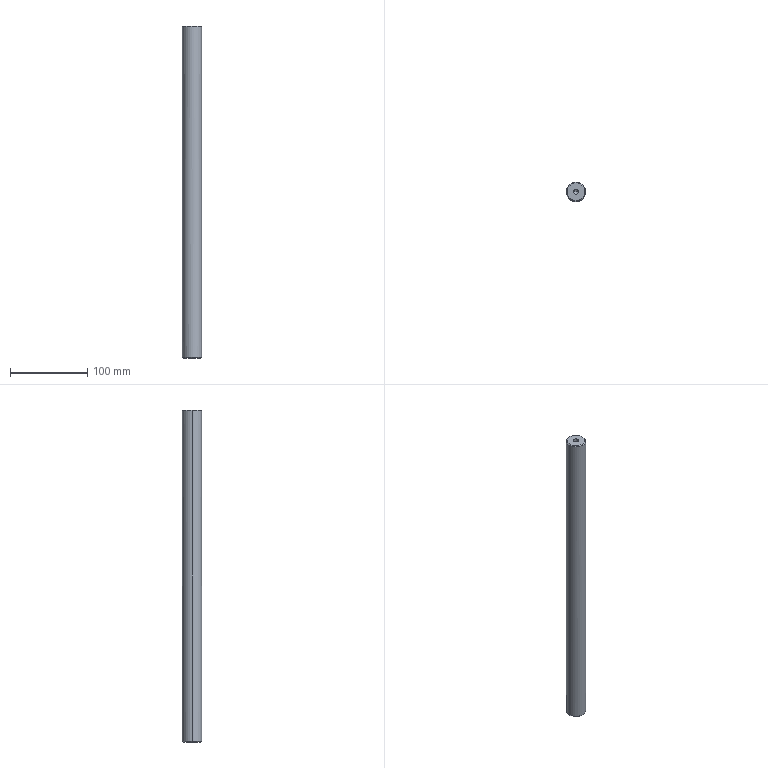Part | STEP file | fBY02F02M-00-20A | 1 solid | 16 faces | box 25 x 25 x 430 mm | volume 209515 mm3 | cone 8 | cylinder 6 | plane 2 | commonest cylinder face diameters 6.8 x4 25 x2
STEP:
#1=CARTESIAN_POINT('',(0.,0.,0.));
#2=DIRECTION('',(0.,0.,1.));
#3=DIRECTION('',(1.,0.,0.));
#4=AXIS2_PLACEMENT_3D('',#1,#2,#3);
#5=CARTESIAN_POINT('',(0.,12.5,429.));
#6=VERTEX_POINT('',#5);
#7=CARTESIAN_POINT('',(12.5,0.,429.));
#8=VERTEX_POINT('',#7);
#9=CARTESIAN_POINT('',(0.,0.,429.));
#10=DIRECTION('',(0.,0.,-1.));
#11=DIRECTION('',(-1.,0.,0.));
#12=AXIS2_PLACEMENT_3D('',#9,#10,#11);
#13=CIRCLE('',#12,12.5);
#14=CARTESIAN_POINT('',(0.,0.,430.));
#15=DIRECTION('',(0.,0.,-1.));
#16=DIRECTION('',(-1.,0.,0.));
#17=AXIS2_PLACEMENT_3D('',#14,#15,#16);
#18=CYLINDRICAL_SURFACE('',#17,12.5);
#19=CARTESIAN_POINT('',(0.,1.));
#20=DIRECTION('',(1.,0.));
#21=VECTOR('',#20,1.);
#22=LINE('',#19,#21);
#23=(GEOMETRIC_REPRESENTATION_CONTEXT(2)PARAMETRIC_REPRESENTATION_CONTEXT()REPRESENTATION_CONTEXT('',''));
#24=DEFINITIONAL_REPRESENTATION('',(#22),#23);
#25=PCURVE('',#18,#24);
#26=CARTESIAN_POINT('',(0.,0.,429.));
#27=DIRECTION('',(0.,0.,-1.));
#28=DIRECTION('',(0.,1.,0.));
#29=AXIS2_PLACEMENT_3D('',#26,#27,#28);
#30=CONICAL_SURFACE('',#29,12.5,0.7854);
#31=CARTESIAN_POINT('',(-1.571,0.));
#32=DIRECTION('',(1.,0.));
#33=VECTOR('',#32,1.);
#34=LINE('',#31,#33);
#35=(GEOMETRIC_REPRESENTATION_CONTEXT(2)PARAMETRIC_REPRESENTATION_CONTEXT()REPRESENTATION_CONTEXT('',''));
#36=DEFINITIONAL_REPRESENTATION('',(#34),#35);
#37=PCURVE('',#30,#36);
#38=SURFACE_CURVE('',#13,(#25,#37),.PCURVE_S1.);
#39=EDGE_CURVE('',#6,#8,#38,.T.);
#40=ORIENTED_EDGE('',*,*,#39,.T.);
#41=CARTESIAN_POINT('',(12.5,0.,1.));
#42=VERTEX_POINT('',#41);
#43=CARTESIAN_POINT('',(12.5,0.,430.));
#44=DIRECTION('',(0.,0.,-1.));
#45=VECTOR('',#44,1.);
#46=LINE('',#43,#45);
#47=CARTESIAN_POINT('',(3.142,0.));
#48=DIRECTION('',(0.,1.));
#49=VECTOR('',#48,1.);
#50=LINE('',#47,#49);
#51=(GEOMETRIC_REPRESENTATION_CONTEXT(2)PARAMETRIC_REPRESENTATION_CONTEXT()REPRESENTATION_CONTEXT('',''));
#52=DEFINITIONAL_REPRESENTATION('',(#50),#51);
#53=PCURVE('',#18,#52);
#54=CARTESIAN_POINT('',(0.,0.,430.));
#55=DIRECTION('',(0.,0.,-1.));
#56=DIRECTION('',(-1.,0.,0.));
#57=AXIS2_PLACEMENT_3D('',#54,#55,#56);
#58=CYLINDRICAL_SURFACE('',#57,12.5);
#59=CARTESIAN_POINT('',(3.142,0.));
#60=DIRECTION('',(0.,1.));
#61=VECTOR('',#60,1.);
#62=LINE('',#59,#61);
#63=(GEOMETRIC_REPRESENTATION_CONTEXT(2)PARAMETRIC_REPRESENTATION_CONTEXT()REPRESENTATION_CONTEXT('',''));
#64=DEFINITIONAL_REPRESENTATION('',(#62),#63);
#65=PCURVE('',#58,#64);
#66=SURFACE_CURVE('',#46,(#53,#65),.PCURVE_S1.);
#67=EDGE_CURVE('',#8,#42,#66,.T.);
#68=ORIENTED_EDGE('',*,*,#67,.T.);
#69=CARTESIAN_POINT('',(-12.5,0.,1.));
#70=VERTEX_POINT('',#69);
#71=CARTESIAN_POINT('',(0.,0.,1.));
#72=DIRECTION('',(0.,0.,1.));
#73=DIRECTION('',(-1.,0.,0.));
#74=AXIS2_PLACEMENT_3D('',#71,#72,#73);
#75=CIRCLE('',#74,12.5);
#76=CARTESIAN_POINT('',(6.283,429.));
#77=DIRECTION('',(-1.,0.));
#78=VECTOR('',#77,1.);
#79=LINE('',#76,#78);
#80=(GEOMETRIC_REPRESENTATION_CONTEXT(2)PARAMETRIC_REPRESENTATION_CONTEXT()REPRESENTATION_CONTEXT('',''));
#81=DEFINITIONAL_REPRESENTATION('',(#79),#80);
#82=PCURVE('',#18,#81);
#83=CARTESIAN_POINT('',(0.,0.,1.));
#84=DIRECTION('',(0.,0.,1.));
#85=DIRECTION('',(1.,0.,0.));
#86=AXIS2_PLACEMENT_3D('',#83,#84,#85);
#87=CONICAL_SURFACE('',#86,12.5,0.7854);
#88=CARTESIAN_POINT('',(-3.142,0.));
#89=DIRECTION('',(1.,0.));
#90=VECTOR('',#89,1.);
#91=LINE('',#88,#90);
#92=(GEOMETRIC_REPRESENTATION_CONTEXT(2)PARAMETRIC_REPRESENTATION_CONTEXT()REPRESENTATION_CONTEXT('',''));
#93=DEFINITIONAL_REPRESENTATION('',(#91),#92);
#94=PCURVE('',#87,#93);
#95=SURFACE_CURVE('',#75,(#82,#94),.PCURVE_S1.);
#96=EDGE_CURVE('',#42,#70,#95,.T.);
#97=ORIENTED_EDGE('',*,*,#96,.T.);
#98=CARTESIAN_POINT('',(-12.5,0.,429.));
#99=VERTEX_POINT('',#98);
#100=CARTESIAN_POINT('',(-12.5,0.,430.));
#101=DIRECTION('',(0.,0.,-1.));
#102=VECTOR('',#101,1.);
#103=LINE('',#100,#102);
#104=CARTESIAN_POINT('',(0.,0.));
#105=DIRECTION('',(0.,1.));
#106=VECTOR('',#105,1.);
#107=LINE('',#104,#106);
#108=(GEOMETRIC_REPRESENTATION_CONTEXT(2)PARAMETRIC_REPRESENTATION_CONTEXT()REPRESENTATION_CONTEXT('',''));
#109=DEFINITIONAL_REPRESENTATION('',(#107),#108);
#110=PCURVE('',#18,#109);
#111=CARTESIAN_POINT('',(6.283,0.));
#112=DIRECTION('',(0.,1.));
#113=VECTOR('',#112,1.);
#114=LINE('',#111,#113);
#115=(GEOMETRIC_REPRESENTATION_CONTEXT(2)PARAMETRIC_REPRESENTATION_CONTEXT()REPRESENTATION_CONTEXT('',''));
#116=DEFINITIONAL_REPRESENTATION('',(#114),#115);
#117=PCURVE('',#58,#116);
#118=SURFACE_CURVE('',#103,(#110,#117),.PCURVE_S1.);
#119=EDGE_CURVE('',#99,#70,#118,.T.);
#120=ORIENTED_EDGE('',*,*,#119,.F.);
#121=CARTESIAN_POINT('',(0.,0.,429.));
#122=DIRECTION('',(0.,0.,-1.));
#123=DIRECTION('',(-1.,0.,0.));
#124=AXIS2_PLACEMENT_3D('',#121,#122,#123);
#125=CIRCLE('',#124,12.5);
#126=CARTESIAN_POINT('',(0.,1.));
#127=DIRECTION('',(1.,0.));
#128=VECTOR('',#127,1.);
#129=LINE('',#126,#128);
#130=(GEOMETRIC_REPRESENTATION_CONTEXT(2)PARAMETRIC_REPRESENTATION_CONTEXT()REPRESENTATION_CONTEXT('',''));
#131=DEFINITIONAL_REPRESENTATION('',(#129),#130);
#132=PCURVE('',#18,#131);
#133=CARTESIAN_POINT('',(0.,0.,429.));
#134=DIRECTION('',(0.,0.,-1.));
#135=DIRECTION('',(0.,1.,0.));
#136=AXIS2_PLACEMENT_3D('',#133,#134,#135);
#137=CONICAL_SURFACE('',#136,12.5,0.7854);
#138=CARTESIAN_POINT('',(4.712,0.));
#139=DIRECTION('',(1.,0.));
#140=VECTOR('',#139,1.);
#141=LINE('',#138,#140);
#142=(GEOMETRIC_REPRESENTATION_CONTEXT(2)PARAMETRIC_REPRESENTATION_CONTEXT()REPRESENTATION_CONTEXT('',''));
#143=DEFINITIONAL_REPRESENTATION('',(#141),#142);
#144=PCURVE('',#137,#143);
#145=SURFACE_CURVE('',#125,(#132,#144),.PCURVE_S1.);
#146=EDGE_CURVE('',#99,#6,#145,.T.);
#147=ORIENTED_EDGE('',*,*,#146,.T.);
#148=EDGE_LOOP('',(#40,#68,#97,#120,#147));
#149=FACE_BOUND('',#148,.T.);
#150=ADVANCED_FACE('',(#149),#18,.T.);
#151=CARTESIAN_POINT('',(11.5,0.,0.));
#152=VERTEX_POINT('',#151);
#153=CARTESIAN_POINT('',(-11.5,0.,0.));
#154=VERTEX_POINT('',#153);
#155=CARTESIAN_POINT('',(0.,0.,0.));
#156=DIRECTION('',(0.,0.,1.));
#157=DIRECTION('',(1.,0.,0.));
#158=AXIS2_PLACEMENT_3D('',#155,#156,#157);
#159=CIRCLE('',#158,11.5);
#160=CARTESIAN_POINT('',(0.,-1.));
#161=DIRECTION('',(1.,0.));
#162=VECTOR('',#161,1.);
#163=LINE('',#160,#162);
#164=(GEOMETRIC_REPRESENTATION_CONTEXT(2)PARAMETRIC_REPRESENTATION_CONTEXT()REPRESENTATION_CONTEXT('',''));
#165=DEFINITIONAL_REPRESENTATION('',(#163),#164);
#166=PCURVE('',#87,#165);
#167=CARTESIAN_POINT('',(0.,0.,0.));
#168=DIRECTION('',(0.,0.,1.));
#169=DIRECTION('',(1.,0.,0.));
#170=AXIS2_PLACEMENT_3D('',#167,#168,#169);
#171=PLANE('',#170);
#172=CARTESIAN_POINT('',(0.,0.));
#173=DIRECTION('',(1.,0.));
#174=AXIS2_PLACEMENT_2D('',#172,#173);
#175=CIRCLE('',#174,11.5);
#176=(GEOMETRIC_REPRESENTATION_CONTEXT(2)PARAMETRIC_REPRESENTATION_CONTEXT()REPRESENTATION_CONTEXT('',''));
#177=DEFINITIONAL_REPRESENTATION('',(#175),#176);
#178=PCURVE('',#171,#177);
#179=SURFACE_CURVE('',#159,(#166,#178),.PCURVE_S1.);
#180=EDGE_CURVE('',#152,#154,#179,.T.);
#181=ORIENTED_EDGE('',*,*,#180,.T.);
#182=CARTESIAN_POINT('',(-12.5,0.,1.));
#183=DIRECTION('',(-0.7071,0.,0.7071));
#184=VECTOR('',#183,1.);
#185=LINE('',#182,#184);
#186=CARTESIAN_POINT('',(3.142,0.));
#187=DIRECTION('',(0.,1.));
#188=VECTOR('',#187,1.);
#189=LINE('',#186,#188);
#190=(GEOMETRIC_REPRESENTATION_CONTEXT(2)PARAMETRIC_REPRESENTATION_CONTEXT()REPRESENTATION_CONTEXT('',''));
#191=DEFINITIONAL_REPRESENTATION('',(#189),#190);
#192=PCURVE('',#87,#191);
#193=CARTESIAN_POINT('',(0.,0.,1.));
#194=DIRECTION('',(0.,0.,1.));
#195=DIRECTION('',(1.,0.,0.));
#196=AXIS2_PLACEMENT_3D('',#193,#194,#195);
#197=CONICAL_SURFACE('',#196,12.5,0.7854);
#198=CARTESIAN_POINT('',(3.142,0.));
#199=DIRECTION('',(0.,1.));
#200=VECTOR('',#199,1.);
#201=LINE('',#198,#200);
#202=(GEOMETRIC_REPRESENTATION_CONTEXT(2)PARAMETRIC_REPRESENTATION_CONTEXT()REPRESENTATION_CONTEXT('',''));
#203=DEFINITIONAL_REPRESENTATION('',(#201),#202);
#204=PCURVE('',#197,#203);
#205=SURFACE_CURVE('',#185,(#192,#204),.PCURVE_S1.);
#206=EDGE_CURVE('',#154,#70,#205,.T.);
#207=ORIENTED_EDGE('',*,*,#206,.T.);
#208=ORIENTED_EDGE('',*,*,#96,.F.);
#209=CARTESIAN_POINT('',(12.5,0.,1.));
#210=DIRECTION('',(0.7071,0.,0.7071));
#211=VECTOR('',#210,1.);
#212=LINE('',#209,#211);
#213=CARTESIAN_POINT('',(0.,0.));
#214=DIRECTION('',(0.,1.));
#215=VECTOR('',#214,1.);
#216=LINE('',#213,#215);
#217=(GEOMETRIC_REPRESENTATION_CONTEXT(2)PARAMETRIC_REPRESENTATION_CONTEXT()REPRESENTATION_CONTEXT('',''));
#218=DEFINITIONAL_REPRESENTATION('',(#216),#217);
#219=PCURVE('',#87,#218);
#220=CARTESIAN_POINT('',(6.283,0.));
#221=DIRECTION('',(0.,1.));
#222=VECTOR('',#221,1.);
#223=LINE('',#220,#222);
#224=(GEOMETRIC_REPRESENTATION_CONTEXT(2)PARAMETRIC_REPRESENTATION_CONTEXT()REPRESENTATION_CONTEXT('',''));
#225=DEFINITIONAL_REPRESENTATION('',(#223),#224);
#226=PCURVE('',#197,#225);
#227=SURFACE_CURVE('',#212,(#219,#226),.PCURVE_S1.);
#228=EDGE_CURVE('',#152,#42,#227,.T.);
#229=ORIENTED_EDGE('',*,*,#228,.F.);
#230=EDGE_LOOP('',(#181,#207,#208,#229));
#231=FACE_BOUND('',#230,.T.);
#232=ADVANCED_FACE('',(#231),#87,.T.);
#233=CARTESIAN_POINT('',(0.,11.5,430.));
#234=VERTEX_POINT('',#233);
#235=CARTESIAN_POINT('',(0.,-11.5,430.));
#236=VERTEX_POINT('',#235);
#237=CARTESIAN_POINT('',(0.,0.,430.));
#238=DIRECTION('',(0.,0.,-1.));
#239=DIRECTION('',(0.,1.,0.));
#240=AXIS2_PLACEMENT_3D('',#237,#238,#239);
#241=CIRCLE('',#240,11.5);
#242=CARTESIAN_POINT('',(0.,-1.));
#243=DIRECTION('',(1.,0.));
#244=VECTOR('',#243,1.);
#245=LINE('',#242,#244);
#246=(GEOMETRIC_REPRESENTATION_CONTEXT(2)PARAMETRIC_REPRESENTATION_CONTEXT()REPRESENTATION_CONTEXT('',''));
#247=DEFINITIONAL_REPRESENTATION('',(#245),#246);
#248=PCURVE('',#30,#247);
#249=CARTESIAN_POINT('',(0.,0.,430.));
#250=DIRECTION('',(0.,0.,1.));
#251=DIRECTION('',(1.,0.,0.));
#252=AXIS2_PLACEMENT_3D('',#249,#250,#251);
#253=PLANE('',#252);
#254=CARTESIAN_POINT('',(0.,11.5));
#255=CARTESIAN_POINT('',(19.919,11.5));
#256=CARTESIAN_POINT('',(9.959,-5.75));
#257=CARTESIAN_POINT('',(0.,-23.));
#258=CARTESIAN_POINT('',(-9.959,-5.75));
#259=CARTESIAN_POINT('',(-19.919,11.5));
#260=CARTESIAN_POINT('',(0.,11.5));
#261=(BOUNDED_CURVE()B_SPLINE_CURVE(2,(#254,#255,#256,#257,#258,#259,#260),.UNSPECIFIED.,.T.,.F.)B_SPLINE_CURVE_WITH_KNOTS((1,2,2,2,2,1),(-2.094,0.,2.094,4.189,6.283,8.378),.UNSPECIFIED.)CURVE()GEOMETRIC_REPRESENTATION_ITEM()RATIONAL_B_SPLINE_CURVE((1.,0.5,1.,0.5,1.,0.5,1.))REPRESENTATION_ITEM(''));
#262=(GEOMETRIC_REPRESENTATION_CONTEXT(2)PARAMETRIC_REPRESENTATION_CONTEXT()REPRESENTATION_CONTEXT('',''));
#263=DEFINITIONAL_REPRESENTATION('',(#261),#262);
#264=PCURVE('',#253,#263);
#265=SURFACE_CURVE('',#241,(#248,#264),.PCURVE_S1.);
#266=EDGE_CURVE('',#234,#236,#265,.T.);
#267=ORIENTED_EDGE('',*,*,#266,.T.);
#268=CARTESIAN_POINT('',(0.,-12.5,429.));
#269=VERTEX_POINT('',#268);
#270=CARTESIAN_POINT('',(0.,-12.5,429.));
#271=DIRECTION('',(0.,-0.7071,-0.7071));
#272=VECTOR('',#271,1.);
#273=LINE('',#270,#272);
#274=CARTESIAN_POINT('',(3.142,0.));
#275=DIRECTION('',(0.,1.));
#276=VECTOR('',#275,1.);
#277=LINE('',#274,#276);
#278=(GEOMETRIC_REPRESENTATION_CONTEXT(2)PARAMETRIC_REPRESENTATION_CONTEXT()REPRESENTATION_CONTEXT('',''));
#279=DEFINITIONAL_REPRESENTATION('',(#277),#278);
#280=PCURVE('',#30,#279);
#281=CARTESIAN_POINT('',(3.142,0.));
#282=DIRECTION('',(0.,1.));
#283=VECTOR('',#282,1.);
#284=LINE('',#281,#283);
#285=(GEOMETRIC_REPRESENTATION_CONTEXT(2)PARAMETRIC_REPRESENTATION_CONTEXT()REPRESENTATION_CONTEXT('',''));
#286=DEFINITIONAL_REPRESENTATION('',(#284),#285);
#287=PCURVE('',#137,#286);
#288=SURFACE_CURVE('',#273,(#280,#287),.PCURVE_S1.);
#289=EDGE_CURVE('',#236,#269,#288,.T.);
#290=ORIENTED_EDGE('',*,*,#289,.T.);
#291=CARTESIAN_POINT('',(0.,0.,429.));
#292=DIRECTION('',(0.,0.,-1.));
#293=DIRECTION('',(-1.,0.,0.));
#294=AXIS2_PLACEMENT_3D('',#291,#292,#293);
#295=CIRCLE('',#294,12.5);
#296=CARTESIAN_POINT('',(-1.571,0.));
#297=DIRECTION('',(1.,0.));
#298=VECTOR('',#297,1.);
#299=LINE('',#296,#298);
#300=(GEOMETRIC_REPRESENTATION_CONTEXT(2)PARAMETRIC_REPRESENTATION_CONTEXT()REPRESENTATION_CONTEXT('',''));
#301=DEFINITIONAL_REPRESENTATION('',(#299),#300);
#302=PCURVE('',#30,#301);
#303=CARTESIAN_POINT('',(0.,1.));
#304=DIRECTION('',(1.,0.));
#305=VECTOR('',#304,1.);
#306=LINE('',#303,#305);
#307=(GEOMETRIC_REPRESENTATION_CONTEXT(2)PARAMETRIC_REPRESENTATION_CONTEXT()REPRESENTATION_CONTEXT('',''));
#308=DEFINITIONAL_REPRESENTATION('',(#306),#307);
#309=PCURVE('',#58,#308);
#310=SURFACE_CURVE('',#295,(#302,#309),.PCURVE_S1.);
#311=EDGE_CURVE('',#8,#269,#310,.T.);
#312=ORIENTED_EDGE('',*,*,#311,.F.);
#313=ORIENTED_EDGE('',*,*,#39,.F.);
#314=CARTESIAN_POINT('',(0.,12.5,429.));
#315=DIRECTION('',(0.,0.7071,-0.7071));
#316=VECTOR('',#315,1.);
#317=LINE('',#314,#316);
#318=CARTESIAN_POINT('',(0.,0.));
#319=DIRECTION('',(0.,1.));
#320=VECTOR('',#319,1.);
#321=LINE('',#318,#320);
#322=(GEOMETRIC_REPRESENTATION_CONTEXT(2)PARAMETRIC_REPRESENTATION_CONTEXT()REPRESENTATION_CONTEXT('',''));
#323=DEFINITIONAL_REPRESENTATION('',(#321),#322);
#324=PCURVE('',#30,#323);
#325=CARTESIAN_POINT('',(6.283,0.));
#326=DIRECTION('',(0.,1.));
#327=VECTOR('',#326,1.);
#328=LINE('',#325,#327);
#329=(GEOMETRIC_REPRESENTATION_CONTEXT(2)PARAMETRIC_REPRESENTATION_CONTEXT()REPRESENTATION_CONTEXT('',''));
#330=DEFINITIONAL_REPRESENTATION('',(#328),#329);
#331=PCURVE('',#137,#330);
#332=SURFACE_CURVE('',#317,(#324,#331),.PCURVE_S1.);
#333=EDGE_CURVE('',#234,#6,#332,.T.);
#334=ORIENTED_EDGE('',*,*,#333,.F.);
#335=EDGE_LOOP('',(#267,#290,#312,#313,#334));
#336=FACE_BOUND('',#335,.T.);
#337=ADVANCED_FACE('',(#336),#30,.T.);
#338=CARTESIAN_POINT('',(-3.4,0.,19.75));
#339=VERTEX_POINT('',#338);
#340=CARTESIAN_POINT('',(-3.4,0.,0.));
#341=VERTEX_POINT('',#340);
#342=CARTESIAN_POINT('',(-3.4,0.,0.));
#343=DIRECTION('',(0.,0.,-1.));
#344=VECTOR('',#343,1.);
#345=LINE('',#342,#344);
#346=CARTESIAN_POINT('',(0.,0.,0.));
#347=DIRECTION('',(0.,0.,-1.));
#348=DIRECTION('',(-1.,0.,0.));
#349=AXIS2_PLACEMENT_3D('',#346,#347,#348);
#350=CYLINDRICAL_SURFACE('',#349,3.4);
#351=CARTESIAN_POINT('',(6.283,0.));
#352=DIRECTION('',(0.,1.));
#353=VECTOR('',#352,1.);
#354=LINE('',#351,#353);
#355=(GEOMETRIC_REPRESENTATION_CONTEXT(2)PARAMETRIC_REPRESENTATION_CONTEXT()REPRESENTATION_CONTEXT('',''));
#356=DEFINITIONAL_REPRESENTATION('',(#354),#355);
#357=PCURVE('',#350,#356);
#358=CARTESIAN_POINT('',(0.,0.,0.));
#359=DIRECTION('',(0.,0.,-1.));
#360=DIRECTION('',(-1.,0.,0.));
#361=AXIS2_PLACEMENT_3D('',#358,#359,#360);
#362=CYLINDRICAL_SURFACE('',#361,3.4);
#363=CARTESIAN_POINT('',(0.,0.));
#364=DIRECTION('',(0.,1.));
#365=VECTOR('',#364,1.);
#366=LINE('',#363,#365);
#367=(GEOMETRIC_REPRESENTATION_CONTEXT(2)PARAMETRIC_REPRESENTATION_CONTEXT()REPRESENTATION_CONTEXT('',''));
#368=DEFINITIONAL_REPRESENTATION('',(#366),#367);
#369=PCURVE('',#362,#368);
#370=SURFACE_CURVE('',#345,(#357,#369),.PCURVE_S1.);
#371=EDGE_CURVE('',#339,#341,#370,.T.);
#372=ORIENTED_EDGE('',*,*,#371,.T.);
#373=CARTESIAN_POINT('',(3.4,0.,0.));
#374=VERTEX_POINT('',#373);
#375=CARTESIAN_POINT('',(0.,0.,0.));
#376=DIRECTION('',(0.,0.,-1.));
#377=DIRECTION('',(-1.,0.,0.));
#378=AXIS2_PLACEMENT_3D('',#375,#376,#377);
#379=CIRCLE('',#378,3.4);
#380=CARTESIAN_POINT('',(0.,0.));
#381=DIRECTION('',(1.,0.));
#382=VECTOR('',#381,1.);
#383=LINE('',#380,#382);
#384=(GEOMETRIC_REPRESENTATION_CONTEXT(2)PARAMETRIC_REPRESENTATION_CONTEXT()REPRESENTATION_CONTEXT('',''));
#385=DEFINITIONAL_REPRESENTATION('',(#383),#384);
#386=PCURVE('',#350,#385);
#387=CARTESIAN_POINT('',(-3.4,0.));
#388=CARTESIAN_POINT('',(-3.4,5.889));
#389=CARTESIAN_POINT('',(1.7,2.944));
#390=CARTESIAN_POINT('',(6.8,0.));
#391=CARTESIAN_POINT('',(1.7,-2.944));
#392=CARTESIAN_POINT('',(-3.4,-5.889));
#393=CARTESIAN_POINT('',(-3.4,0.));
#394=(BOUNDED_CURVE()B_SPLINE_CURVE(2,(#387,#388,#389,#390,#391,#392,#393),.UNSPECIFIED.,.T.,.F.)B_SPLINE_CURVE_WITH_KNOTS((1,2,2,2,2,1),(-2.094,0.,2.094,4.189,6.283,8.378),.UNSPECIFIED.)CURVE()GEOMETRIC_REPRESENTATION_ITEM()RATIONAL_B_SPLINE_CURVE((1.,0.5,1.,0.5,1.,0.5,1.))REPRESENTATION_ITEM(''));
#395=(GEOMETRIC_REPRESENTATION_CONTEXT(2)PARAMETRIC_REPRESENTATION_CONTEXT()REPRESENTATION_CONTEXT('',''));
#396=DEFINITIONAL_REPRESENTATION('',(#394),#395);
#397=PCURVE('',#171,#396);
#398=SURFACE_CURVE('',#379,(#386,#397),.PCURVE_S1.);
#399=EDGE_CURVE('',#374,#341,#398,.T.);
#400=ORIENTED_EDGE('',*,*,#399,.F.);
#401=CARTESIAN_POINT('',(3.4,0.,19.75));
#402=VERTEX_POINT('',#401);
#403=CARTESIAN_POINT('',(3.4,0.,0.));
#404=DIRECTION('',(0.,0.,-1.));
#405=VECTOR('',#404,1.);
#406=LINE('',#403,#405);
#407=CARTESIAN_POINT('',(3.142,0.));
#408=DIRECTION('',(0.,1.));
#409=VECTOR('',#408,1.);
#410=LINE('',#407,#409);
#411=(GEOMETRIC_REPRESENTATION_CONTEXT(2)PARAMETRIC_REPRESENTATION_CONTEXT()REPRESENTATION_CONTEXT('',''));
#412=DEFINITIONAL_REPRESENTATION('',(#410),#411);
#413=PCURVE('',#350,#412);
#414=CARTESIAN_POINT('',(3.142,0.));
#415=DIRECTION('',(0.,1.));
#416=VECTOR('',#415,1.);
#417=LINE('',#414,#416);
#418=(GEOMETRIC_REPRESENTATION_CONTEXT(2)PARAMETRIC_REPRESENTATION_CONTEXT()REPRESENTATION_CONTEXT('',''));
#419=DEFINITIONAL_REPRESENTATION('',(#417),#418);
#420=PCURVE('',#362,#419);
#421=SURFACE_CURVE('',#406,(#413,#420),.PCURVE_S1.);
#422=EDGE_CURVE('',#402,#374,#421,.T.);
#423=ORIENTED_EDGE('',*,*,#422,.F.);
#424=CARTESIAN_POINT('',(0.,0.,19.75));
#425=DIRECTION('',(0.,0.,-1.));
#426=DIRECTION('',(-1.,0.,0.));
#427=AXIS2_PLACEMENT_3D('',#424,#425,#426);
#428=CIRCLE('',#427,3.4);
#429=CARTESIAN_POINT('',(0.,-19.75));
#430=DIRECTION('',(1.,0.));
#431=VECTOR('',#430,1.);
#432=LINE('',#429,#431);
#433=(GEOMETRIC_REPRESENTATION_CONTEXT(2)PARAMETRIC_REPRESENTATION_CONTEXT()REPRESENTATION_CONTEXT('',''));
#434=DEFINITIONAL_REPRESENTATION('',(#432),#433);
#435=PCURVE('',#350,#434);
#436=CARTESIAN_POINT('',(0.,0.,19.75));
#437=DIRECTION('',(0.,0.,-1.));
#438=DIRECTION('',(-1.,0.,0.));
#439=AXIS2_PLACEMENT_3D('',#436,#437,#438);
#440=CONICAL_SURFACE('',#439,3.4,1.03);
#441=CARTESIAN_POINT('',(0.,0.));
#442=DIRECTION('',(1.,0.));
#443=VECTOR('',#442,1.);
#444=LINE('',#441,#443);
#445=(GEOMETRIC_REPRESENTATION_CONTEXT(2)PARAMETRIC_REPRESENTATION_CONTEXT()REPRESENTATION_CONTEXT('',''));
#446=DEFINITIONAL_REPRESENTATION('',(#444),#445);
#447=PCURVE('',#440,#446);
#448=SURFACE_CURVE('',#428,(#435,#447),.PCURVE_S1.);
#449=EDGE_CURVE('',#402,#339,#448,.T.);
#450=ORIENTED_EDGE('',*,*,#449,.T.);
#451=EDGE_LOOP('',(#372,#400,#423,#450));
#452=FACE_BOUND('',#451,.F.);
#453=ADVANCED_FACE('',(#452),#350,.F.);
#454=CARTESIAN_POINT('',(3.4,0.,410.25));
#455=VERTEX_POINT('',#454);
#456=CARTESIAN_POINT('',(3.4,0.,430.));
#457=VERTEX_POINT('',#456);
#458=CARTESIAN_POINT('',(3.4,0.,430.));
#459=DIRECTION('',(0.,0.,1.));
#460=VECTOR('',#459,1.);
#461=LINE('',#458,#460);
#462=CARTESIAN_POINT('',(0.,0.,430.));
#463=DIRECTION('',(0.,0.,1.));
#464=DIRECTION('',(1.,0.,0.));
#465=AXIS2_PLACEMENT_3D('',#462,#463,#464);
#466=CYLINDRICAL_SURFACE('',#465,3.4);
#467=CARTESIAN_POINT('',(6.283,0.));
#468=DIRECTION('',(0.,1.));
#469=VECTOR('',#468,1.);
#470=LINE('',#467,#469);
#471=(GEOMETRIC_REPRESENTATION_CONTEXT(2)PARAMETRIC_REPRESENTATION_CONTEXT()REPRESENTATION_CONTEXT('',''));
#472=DEFINITIONAL_REPRESENTATION('',(#470),#471);
#473=PCURVE('',#466,#472);
#474=CARTESIAN_POINT('',(0.,0.,430.));
#475=DIRECTION('',(0.,0.,1.));
#476=DIRECTION('',(1.,0.,0.));
#477=AXIS2_PLACEMENT_3D('',#474,#475,#476);
#478=CYLINDRICAL_SURFACE('',#477,3.4);
#479=CARTESIAN_POINT('',(0.,0.));
#480=DIRECTION('',(0.,1.));
#481=VECTOR('',#480,1.);
#482=LINE('',#479,#481);
#483=(GEOMETRIC_REPRESENTATION_CONTEXT(2)PARAMETRIC_REPRESENTATION_CONTEXT()REPRESENTATION_CONTEXT('',''));
#484=DEFINITIONAL_REPRESENTATION('',(#482),#483);
#485=PCURVE('',#478,#484);
#486=SURFACE_CURVE('',#461,(#473,#485),.PCURVE_S1.);
#487=EDGE_CURVE('',#455,#457,#486,.T.);
#488=ORIENTED_EDGE('',*,*,#487,.T.);
#489=CARTESIAN_POINT('',(-3.4,0.,430.));
#490=VERTEX_POINT('',#489);
#491=CARTESIAN_POINT('',(0.,0.,430.));
#492=DIRECTION('',(0.,0.,-1.));
#493=DIRECTION('',(1.,0.,0.));
#494=AXIS2_PLACEMENT_3D('',#491,#492,#493);
#495=CIRCLE('',#494,3.4);
#496=CARTESIAN_POINT('',(6.283,0.));
#497=DIRECTION('',(-1.,0.));
#498=VECTOR('',#497,1.);
#499=LINE('',#496,#498);
#500=(GEOMETRIC_REPRESENTATION_CONTEXT(2)PARAMETRIC_REPRESENTATION_CONTEXT()REPRESENTATION_CONTEXT('',''));
#501=DEFINITIONAL_REPRESENTATION('',(#499),#500);
#502=PCURVE('',#466,#501);
#503=CARTESIAN_POINT('',(3.4,0.));
#504=CARTESIAN_POINT('',(3.4,-5.889));
#505=CARTESIAN_POINT('',(-1.7,-2.944));
#506=CARTESIAN_POINT('',(-6.8,0.));
#507=CARTESIAN_POINT('',(-1.7,2.944));
#508=CARTESIAN_POINT('',(3.4,5.889));
#509=CARTESIAN_POINT('',(3.4,0.));
#510=(BOUNDED_CURVE()B_SPLINE_CURVE(2,(#503,#504,#505,#506,#507,#508,#509),.UNSPECIFIED.,.T.,.F.)B_SPLINE_CURVE_WITH_KNOTS((1,2,2,2,2,1),(-2.094,0.,2.094,4.189,6.283,8.378),.UNSPECIFIED.)CURVE()GEOMETRIC_REPRESENTATION_ITEM()RATIONAL_B_SPLINE_CURVE((1.,0.5,1.,0.5,1.,0.5,1.))REPRESENTATION_ITEM(''));
#511=(GEOMETRIC_REPRESENTATION_CONTEXT(2)PARAMETRIC_REPRESENTATION_CONTEXT()REPRESENTATION_CONTEXT('',''));
#512=DEFINITIONAL_REPRESENTATION('',(#510),#511);
#513=PCURVE('',#253,#512);
#514=SURFACE_CURVE('',#495,(#502,#513),.PCURVE_S1.);
#515=EDGE_CURVE('',#457,#490,#514,.T.);
#516=ORIENTED_EDGE('',*,*,#515,.T.);
#517=CARTESIAN_POINT('',(-3.4,0.,410.25));
#518=VERTEX_POINT('',#517);
#519=CARTESIAN_POINT('',(-3.4,0.,430.));
#520=DIRECTION('',(0.,0.,1.));
#521=VECTOR('',#520,1.);
#522=LINE('',#519,#521);
#523=CARTESIAN_POINT('',(3.142,0.));
#524=DIRECTION('',(0.,1.));
#525=VECTOR('',#524,1.);
#526=LINE('',#523,#525);
#527=(GEOMETRIC_REPRESENTATION_CONTEXT(2)PARAMETRIC_REPRESENTATION_CONTEXT()REPRESENTATION_CONTEXT('',''));
#528=DEFINITIONAL_REPRESENTATION('',(#526),#527);
#529=PCURVE('',#466,#528);
#530=CARTESIAN_POINT('',(3.142,0.));
#531=DIRECTION('',(0.,1.));
#532=VECTOR('',#531,1.);
#533=LINE('',#530,#532);
#534=(GEOMETRIC_REPRESENTATION_CONTEXT(2)PARAMETRIC_REPRESENTATION_CONTEXT()REPRESENTATION_CONTEXT('',''));
#535=DEFINITIONAL_REPRESENTATION('',(#533),#534);
#536=PCURVE('',#478,#535);
#537=SURFACE_CURVE('',#522,(#529,#536),.PCURVE_S1.);
#538=EDGE_CURVE('',#518,#490,#537,.T.);
#539=ORIENTED_EDGE('',*,*,#538,.F.);
#540=CARTESIAN_POINT('',(0.,0.,410.25));
#541=DIRECTION('',(0.,0.,1.));
#542=DIRECTION('',(1.,0.,0.));
#543=AXIS2_PLACEMENT_3D('',#540,#541,#542);
#544=CIRCLE('',#543,3.4);
#545=CARTESIAN_POINT('',(0.,-19.75));
#546=DIRECTION('',(1.,0.));
#547=VECTOR('',#546,1.);
#548=LINE('',#545,#547);
#549=(GEOMETRIC_REPRESENTATION_CONTEXT(2)PARAMETRIC_REPRESENTATION_CONTEXT()REPRESENTATION_CONTEXT('',''));
#550=DEFINITIONAL_REPRESENTATION('',(#548),#549);
#551=PCURVE('',#466,#550);
#552=CARTESIAN_POINT('',(0.,0.,410.25));
#553=DIRECTION('',(0.,0.,1.));
#554=DIRECTION('',(1.,0.,0.));
#555=AXIS2_PLACEMENT_3D('',#552,#553,#554);
#556=CONICAL_SURFACE('',#555,3.4,1.03);
#557=CARTESIAN_POINT('',(0.,0.));
#558=DIRECTION('',(1.,0.));
#559=VECTOR('',#558,1.);
#560=LINE('',#557,#559);
#561=(GEOMETRIC_REPRESENTATION_CONTEXT(2)PARAMETRIC_REPRESENTATION_CONTEXT()REPRESENTATION_CONTEXT('',''));
#562=DEFINITIONAL_REPRESENTATION('',(#560),#561);
#563=PCURVE('',#556,#562);
#564=SURFACE_CURVE('',#544,(#551,#563),.PCURVE_S1.);
#565=EDGE_CURVE('',#518,#455,#564,.T.);
#566=ORIENTED_EDGE('',*,*,#565,.T.);
#567=EDGE_LOOP('',(#488,#516,#539,#566));
#568=FACE_BOUND('',#567,.F.);
#569=ADVANCED_FACE('',(#568),#466,.F.);
#570=ORIENTED_EDGE('',*,*,#449,.F.);
#571=CARTESIAN_POINT('',(0.,0.,21.793));
#572=VERTEX_POINT('',#571);
#573=CARTESIAN_POINT('',(3.4,0.,19.75));
#574=DIRECTION('',(0.8572,0.,-0.515));
#575=VECTOR('',#574,1.);
#576=LINE('',#573,#575);
#577=CARTESIAN_POINT('',(3.142,0.));
#578=DIRECTION('',(0.,1.));
#579=VECTOR('',#578,1.);
#580=LINE('',#577,#579);
#581=(GEOMETRIC_REPRESENTATION_CONTEXT(2)PARAMETRIC_REPRESENTATION_CONTEXT()REPRESENTATION_CONTEXT('',''));
#582=DEFINITIONAL_REPRESENTATION('',(#580),#581);
#583=PCURVE('',#440,#582);
#584=CARTESIAN_POINT('',(0.,0.,19.75));
#585=DIRECTION('',(0.,0.,-1.));
#586=DIRECTION('',(-1.,0.,0.));
#587=AXIS2_PLACEMENT_3D('',#584,#585,#586);
#588=CONICAL_SURFACE('',#587,3.4,1.03);
#589=CARTESIAN_POINT('',(3.142,0.));
#590=DIRECTION('',(0.,1.));
#591=VECTOR('',#590,1.);
#592=LINE('',#589,#591);
#593=(GEOMETRIC_REPRESENTATION_CONTEXT(2)PARAMETRIC_REPRESENTATION_CONTEXT()REPRESENTATION_CONTEXT('',''));
#594=DEFINITIONAL_REPRESENTATION('',(#592),#593);
#595=PCURVE('',#588,#594);
#596=SURFACE_CURVE('',#576,(#583,#595),.PCURVE_S1.);
#597=EDGE_CURVE('',#572,#402,#596,.T.);
#598=ORIENTED_EDGE('',*,*,#597,.F.);
#599=CARTESIAN_POINT('',(-3.4,0.,19.75));
#600=DIRECTION('',(-0.8572,0.,-0.515));
#601=VECTOR('',#600,1.);
#602=LINE('',#599,#601);
#603=CARTESIAN_POINT('',(6.283,0.));
#604=DIRECTION('',(0.,1.));
#605=VECTOR('',#604,1.);
#606=LINE('',#603,#605);
#607=(GEOMETRIC_REPRESENTATION_CONTEXT(2)PARAMETRIC_REPRESENTATION_CONTEXT()REPRESENTATION_CONTEXT('',''));
#608=DEFINITIONAL_REPRESENTATION('',(#606),#607);
#609=PCURVE('',#440,#608);
#610=CARTESIAN_POINT('',(0.,0.));
#611=DIRECTION('',(0.,1.));
#612=VECTOR('',#611,1.);
#613=LINE('',#610,#612);
#614=(GEOMETRIC_REPRESENTATION_CONTEXT(2)PARAMETRIC_REPRESENTATION_CONTEXT()REPRESENTATION_CONTEXT('',''));
#615=DEFINITIONAL_REPRESENTATION('',(#613),#614);
#616=PCURVE('',#588,#615);
#617=SURFACE_CURVE('',#602,(#609,#616),.PCURVE_S1.);
#618=EDGE_CURVE('',#572,#339,#617,.T.);
#619=ORIENTED_EDGE('',*,*,#618,.T.);
#620=EDGE_LOOP('',(#570,#598,#619));
#621=FACE_BOUND('',#620,.F.);
#622=ADVANCED_FACE('',(#621),#440,.F.);
#623=ORIENTED_EDGE('',*,*,#565,.F.);
#624=CARTESIAN_POINT('',(0.,0.,408.207));
#625=VERTEX_POINT('',#624);
#626=CARTESIAN_POINT('',(-3.4,0.,410.25));
#627=DIRECTION('',(-0.8572,0.,0.515));
#628=VECTOR('',#627,1.);
#629=LINE('',#626,#628);
#630=CARTESIAN_POINT('',(3.142,-2.043));
#631=CARTESIAN_POINT('',(3.142,-2.012));
#632=CARTESIAN_POINT('',(3.142,-1.95));
#633=CARTESIAN_POINT('',(3.142,-1.857));
#634=CARTESIAN_POINT('',(3.142,-1.764));
#635=CARTESIAN_POINT('',(3.142,-1.671));
#636=CARTESIAN_POINT('',(3.142,-1.579));
#637=CARTESIAN_POINT('',(3.142,-1.486));
#638=CARTESIAN_POINT('',(3.142,-1.393));
#639=CARTESIAN_POINT('',(3.142,-1.3));
#640=CARTESIAN_POINT('',(3.142,-1.207));
#641=CARTESIAN_POINT('',(3.142,-1.114));
#642=CARTESIAN_POINT('',(3.142,-1.021));
#643=CARTESIAN_POINT('',(3.142,-0.9286));
#644=CARTESIAN_POINT('',(3.142,-0.8357));
#645=CARTESIAN_POINT('',(3.142,-0.7429));
#646=CARTESIAN_POINT('',(3.142,-0.65));
#647=CARTESIAN_POINT('',(3.142,-0.5572));
#648=CARTESIAN_POINT('',(3.142,-0.4643));
#649=CARTESIAN_POINT('',(3.142,-0.3714));
#650=CARTESIAN_POINT('',(3.142,-0.2786));
#651=CARTESIAN_POINT('',(3.142,-0.1857));
#652=CARTESIAN_POINT('',(3.142,-0.09286));
#653=CARTESIAN_POINT('',(3.142,-0.03095));
#654=CARTESIAN_POINT('',(3.142,0.));
#655=B_SPLINE_CURVE_WITH_KNOTS('',3,(#630,#631,#632,#633,#634,#635,#636,#637,#638,#639,#640,#641,#642,#643,#644,#645,#646,#647,#648,#649,#650,#651,#652,#653,#654),.UNSPECIFIED.,.F.,.F.,(4,1,1,1,1,1,1,1,1,1,1,1,1,1,1,1,1,1,1,1,1,1,4),(-3.967,-3.786,-3.606,-3.426,-3.245,-3.065,-2.885,-2.704,-2.524,-2.344,-2.164,-1.983,-1.803,-1.623,-1.442,-1.262,-1.082,-0.9015,-0.7212,-0.5409,-0.3606,-0.1803,0.),.QUASI_UNIFORM_KNOTS.);
#656=(GEOMETRIC_REPRESENTATION_CONTEXT(2)PARAMETRIC_REPRESENTATION_CONTEXT()REPRESENTATION_CONTEXT('',''));
#657=DEFINITIONAL_REPRESENTATION('',(#655),#656);
#658=PCURVE('',#556,#657);
#659=CARTESIAN_POINT('',(0.,0.,410.25));
#660=DIRECTION('',(0.,0.,1.));
#661=DIRECTION('',(1.,0.,0.));
#662=AXIS2_PLACEMENT_3D('',#659,#660,#661);
#663=CONICAL_SURFACE('',#662,3.4,1.03);
#664=CARTESIAN_POINT('',(3.142,-2.043));
#665=CARTESIAN_POINT('',(3.142,-2.012));
#666=CARTESIAN_POINT('',(3.142,-1.95));
#667=CARTESIAN_POINT('',(3.142,-1.857));
#668=CARTESIAN_POINT('',(3.142,-1.764));
#669=CARTESIAN_POINT('',(3.142,-1.671));
#670=CARTESIAN_POINT('',(3.142,-1.579));
#671=CARTESIAN_POINT('',(3.142,-1.486));
#672=CARTESIAN_POINT('',(3.142,-1.393));
#673=CARTESIAN_POINT('',(3.142,-1.3));
#674=CARTESIAN_POINT('',(3.142,-1.207));
#675=CARTESIAN_POINT('',(3.142,-1.114));
#676=CARTESIAN_POINT('',(3.142,-1.021));
#677=CARTESIAN_POINT('',(3.142,-0.9286));
#678=CARTESIAN_POINT('',(3.142,-0.8357));
#679=CARTESIAN_POINT('',(3.142,-0.7429));
#680=CARTESIAN_POINT('',(3.142,-0.65));
#681=CARTESIAN_POINT('',(3.142,-0.5572));
#682=CARTESIAN_POINT('',(3.142,-0.4643));
#683=CARTESIAN_POINT('',(3.142,-0.3714));
#684=CARTESIAN_POINT('',(3.142,-0.2786));
#685=CARTESIAN_POINT('',(3.142,-0.1857));
#686=CARTESIAN_POINT('',(3.142,-0.09286));
#687=CARTESIAN_POINT('',(3.142,-0.03095));
#688=CARTESIAN_POINT('',(3.142,0.));
#689=B_SPLINE_CURVE_WITH_KNOTS('',3,(#664,#665,#666,#667,#668,#669,#670,#671,#672,#673,#674,#675,#676,#677,#678,#679,#680,#681,#682,#683,#684,#685,#686,#687,#688),.UNSPECIFIED.,.F.,.F.,(4,1,1,1,1,1,1,1,1,1,1,1,1,1,1,1,1,1,1,1,1,1,4),(-3.967,-3.786,-3.606,-3.426,-3.245,-3.065,-2.885,-2.704,-2.524,-2.344,-2.164,-1.983,-1.803,-1.623,-1.442,-1.262,-1.082,-0.9015,-0.7212,-0.5409,-0.3606,-0.1803,0.),.QUASI_UNIFORM_KNOTS.);
#690=(GEOMETRIC_REPRESENTATION_CONTEXT(2)PARAMETRIC_REPRESENTATION_CONTEXT()REPRESENTATION_CONTEXT('',''));
#691=DEFINITIONAL_REPRESENTATION('',(#689),#690);
#692=PCURVE('',#663,#691);
#693=SURFACE_CURVE('',#629,(#658,#692),.PCURVE_S1.);
#694=EDGE_CURVE('',#625,#518,#693,.T.);
#695=ORIENTED_EDGE('',*,*,#694,.F.);
#696=CARTESIAN_POINT('',(3.4,0.,410.25));
#697=DIRECTION('',(0.8572,0.,0.515));
#698=VECTOR('',#697,1.);
#699=LINE('',#696,#698);
#700=CARTESIAN_POINT('',(6.283,-2.043));
#701=CARTESIAN_POINT('',(6.283,-2.012));
#702=CARTESIAN_POINT('',(6.283,-1.95));
#703=CARTESIAN_POINT('',(6.283,-1.857));
#704=CARTESIAN_POINT('',(6.283,-1.764));
#705=CARTESIAN_POINT('',(6.283,-1.671));
#706=CARTESIAN_POINT('',(6.283,-1.579));
#707=CARTESIAN_POINT('',(6.283,-1.486));
#708=CARTESIAN_POINT('',(6.283,-1.393));
#709=CARTESIAN_POINT('',(6.283,-1.3));
#710=CARTESIAN_POINT('',(6.283,-1.207));
#711=CARTESIAN_POINT('',(6.283,-1.114));
#712=CARTESIAN_POINT('',(6.283,-1.021));
#713=CARTESIAN_POINT('',(6.283,-0.9286));
#714=CARTESIAN_POINT('',(6.283,-0.8357));
#715=CARTESIAN_POINT('',(6.283,-0.7429));
#716=CARTESIAN_POINT('',(6.283,-0.65));
#717=CARTESIAN_POINT('',(6.283,-0.5572));
#718=CARTESIAN_POINT('',(6.283,-0.4643));
#719=CARTESIAN_POINT('',(6.283,-0.3714));
#720=CARTESIAN_POINT('',(6.283,-0.2786));
#721=CARTESIAN_POINT('',(6.283,-0.1857));
#722=CARTESIAN_POINT('',(6.283,-0.09286));
#723=CARTESIAN_POINT('',(6.283,-0.03095));
#724=CARTESIAN_POINT('',(6.283,0.));
#725=B_SPLINE_CURVE_WITH_KNOTS('',3,(#700,#701,#702,#703,#704,#705,#706,#707,#708,#709,#710,#711,#712,#713,#714,#715,#716,#717,#718,#719,#720,#721,#722,#723,#724),.UNSPECIFIED.,.F.,.F.,(4,1,1,1,1,1,1,1,1,1,1,1,1,1,1,1,1,1,1,1,1,1,4),(-3.967,-3.786,-3.606,-3.426,-3.245,-3.065,-2.885,-2.704,-2.524,-2.344,-2.164,-1.983,-1.803,-1.623,-1.442,-1.262,-1.082,-0.9015,-0.7212,-0.5409,-0.3606,-0.1803,0.),.QUASI_UNIFORM_KNOTS.);
#726=(GEOMETRIC_REPRESENTATION_CONTEXT(2)PARAMETRIC_REPRESENTATION_CONTEXT()REPRESENTATION_CONTEXT('',''));
#727=DEFINITIONAL_REPRESENTATION('',(#725),#726);
#728=PCURVE('',#556,#727);
#729=CARTESIAN_POINT('',(0.,-2.043));
#730=CARTESIAN_POINT('',(0.,-2.012));
#731=CARTESIAN_POINT('',(0.,-1.95));
#732=CARTESIAN_POINT('',(0.,-1.857));
#733=CARTESIAN_POINT('',(0.,-1.764));
#734=CARTESIAN_POINT('',(0.,-1.671));
#735=CARTESIAN_POINT('',(0.,-1.579));
#736=CARTESIAN_POINT('',(0.,-1.486));
#737=CARTESIAN_POINT('',(0.,-1.393));
#738=CARTESIAN_POINT('',(0.,-1.3));
#739=CARTESIAN_POINT('',(0.,-1.207));
#740=CARTESIAN_POINT('',(0.,-1.114));
#741=CARTESIAN_POINT('',(0.,-1.021));
#742=CARTESIAN_POINT('',(0.,-0.9286));
#743=CARTESIAN_POINT('',(0.,-0.8357));
#744=CARTESIAN_POINT('',(0.,-0.7429));
#745=CARTESIAN_POINT('',(0.,-0.65));
#746=CARTESIAN_POINT('',(0.,-0.5572));
#747=CARTESIAN_POINT('',(0.,-0.4643));
#748=CARTESIAN_POINT('',(0.,-0.3714));
#749=CARTESIAN_POINT('',(0.,-0.2786));
#750=CARTESIAN_POINT('',(0.,-0.1857));
#751=CARTESIAN_POINT('',(0.,-0.09286));
#752=CARTESIAN_POINT('',(0.,-0.03095));
#753=CARTESIAN_POINT('',(0.,0.));
#754=B_SPLINE_CURVE_WITH_KNOTS('',3,(#729,#730,#731,#732,#733,#734,#735,#736,#737,#738,#739,#740,#741,#742,#743,#744,#745,#746,#747,#748,#749,#750,#751,#752,#753),.UNSPECIFIED.,.F.,.F.,(4,1,1,1,1,1,1,1,1,1,1,1,1,1,1,1,1,1,1,1,1,1,4),(-3.967,-3.786,-3.606,-3.426,-3.245,-3.065,-2.885,-2.704,-2.524,-2.344,-2.164,-1.983,-1.803,-1.623,-1.442,-1.262,-1.082,-0.9015,-0.7212,-0.5409,-0.3606,-0.1803,0.),.QUASI_UNIFORM_KNOTS.);
#755=(GEOMETRIC_REPRESENTATION_CONTEXT(2)PARAMETRIC_REPRESENTATION_CONTEXT()REPRESENTATION_CONTEXT('',''));
#756=DEFINITIONAL_REPRESENTATION('',(#754),#755);
#757=PCURVE('',#663,#756);
#758=SURFACE_CURVE('',#699,(#728,#757),.PCURVE_S1.);
#759=EDGE_CURVE('',#625,#455,#758,.T.);
#760=ORIENTED_EDGE('',*,*,#759,.T.);
#761=EDGE_LOOP('',(#623,#695,#760));
#762=FACE_BOUND('',#761,.F.);
#763=ADVANCED_FACE('',(#762),#556,.F.);
#764=ORIENTED_EDGE('',*,*,#67,.F.);
#765=ORIENTED_EDGE('',*,*,#311,.T.);
#766=CARTESIAN_POINT('',(0.,0.,429.));
#767=DIRECTION('',(0.,0.,-1.));
#768=DIRECTION('',(-1.,0.,0.));
#769=AXIS2_PLACEMENT_3D('',#766,#767,#768);
#770=CIRCLE('',#769,12.5);
#771=CARTESIAN_POINT('',(0.,1.));
#772=DIRECTION('',(1.,0.));
#773=VECTOR('',#772,1.);
#774=LINE('',#771,#773);
#775=(GEOMETRIC_REPRESENTATION_CONTEXT(2)PARAMETRIC_REPRESENTATION_CONTEXT()REPRESENTATION_CONTEXT('',''));
#776=DEFINITIONAL_REPRESENTATION('',(#774),#775);
#777=PCURVE('',#58,#776);
#778=CARTESIAN_POINT('',(-1.571,0.));
#779=DIRECTION('',(1.,0.));
#780=VECTOR('',#779,1.);
#781=LINE('',#778,#780);
#782=(GEOMETRIC_REPRESENTATION_CONTEXT(2)PARAMETRIC_REPRESENTATION_CONTEXT()REPRESENTATION_CONTEXT('',''));
#783=DEFINITIONAL_REPRESENTATION('',(#781),#782);
#784=PCURVE('',#137,#783);
#785=SURFACE_CURVE('',#770,(#777,#784),.PCURVE_S1.);
#786=EDGE_CURVE('',#269,#99,#785,.T.);
#787=ORIENTED_EDGE('',*,*,#786,.T.);
#788=ORIENTED_EDGE('',*,*,#119,.T.);
#789=CARTESIAN_POINT('',(0.,0.,1.));
#790=DIRECTION('',(0.,0.,1.));
#791=DIRECTION('',(-1.,0.,0.));
#792=AXIS2_PLACEMENT_3D('',#789,#790,#791);
#793=CIRCLE('',#792,12.5);
#794=CARTESIAN_POINT('',(6.283,429.));
#795=DIRECTION('',(-1.,0.));
#796=VECTOR('',#795,1.);
#797=LINE('',#794,#796);
#798=(GEOMETRIC_REPRESENTATION_CONTEXT(2)PARAMETRIC_REPRESENTATION_CONTEXT()REPRESENTATION_CONTEXT('',''));
#799=DEFINITIONAL_REPRESENTATION('',(#797),#798);
#800=PCURVE('',#58,#799);
#801=CARTESIAN_POINT('',(3.142,0.));
#802=DIRECTION('',(1.,0.));
#803=VECTOR('',#802,1.);
#804=LINE('',#801,#803);
#805=(GEOMETRIC_REPRESENTATION_CONTEXT(2)PARAMETRIC_REPRESENTATION_CONTEXT()REPRESENTATION_CONTEXT('',''));
#806=DEFINITIONAL_REPRESENTATION('',(#804),#805);
#807=PCURVE('',#197,#806);
#808=SURFACE_CURVE('',#793,(#800,#807),.PCURVE_S1.);
#809=EDGE_CURVE('',#70,#42,#808,.T.);
#810=ORIENTED_EDGE('',*,*,#809,.T.);
#811=EDGE_LOOP('',(#764,#765,#787,#788,#810));
#812=FACE_BOUND('',#811,.T.);
#813=ADVANCED_FACE('',(#812),#58,.T.);
#814=ORIENTED_EDGE('',*,*,#206,.F.);
#815=CARTESIAN_POINT('',(0.,0.,0.));
#816=DIRECTION('',(0.,0.,1.));
#817=DIRECTION('',(1.,0.,0.));
#818=AXIS2_PLACEMENT_3D('',#815,#816,#817);
#819=CIRCLE('',#818,11.5);
#820=CARTESIAN_POINT('',(0.,-1.));
#821=DIRECTION('',(1.,0.));
#822=VECTOR('',#821,1.);
#823=LINE('',#820,#822);
#824=(GEOMETRIC_REPRESENTATION_CONTEXT(2)PARAMETRIC_REPRESENTATION_CONTEXT()REPRESENTATION_CONTEXT('',''));
#825=DEFINITIONAL_REPRESENTATION('',(#823),#824);
#826=PCURVE('',#197,#825);
#827=CARTESIAN_POINT('',(0.,0.));
#828=DIRECTION('',(1.,0.));
#829=AXIS2_PLACEMENT_2D('',#827,#828);
#830=CIRCLE('',#829,11.5);
#831=(GEOMETRIC_REPRESENTATION_CONTEXT(2)PARAMETRIC_REPRESENTATION_CONTEXT()REPRESENTATION_CONTEXT('',''));
#832=DEFINITIONAL_REPRESENTATION('',(#830),#831);
#833=PCURVE('',#171,#832);
#834=SURFACE_CURVE('',#819,(#826,#833),.PCURVE_S1.);
#835=EDGE_CURVE('',#154,#152,#834,.T.);
#836=ORIENTED_EDGE('',*,*,#835,.T.);
#837=ORIENTED_EDGE('',*,*,#228,.T.);
#838=ORIENTED_EDGE('',*,*,#809,.F.);
#839=EDGE_LOOP('',(#814,#836,#837,#838));
#840=FACE_BOUND('',#839,.T.);
#841=ADVANCED_FACE('',(#840),#197,.T.);
#842=ORIENTED_EDGE('',*,*,#289,.F.);
#843=CARTESIAN_POINT('',(0.,0.,430.));
#844=DIRECTION('',(0.,0.,-1.));
#845=DIRECTION('',(0.,1.,0.));
#846=AXIS2_PLACEMENT_3D('',#843,#844,#845);
#847=CIRCLE('',#846,11.5);
#848=CARTESIAN_POINT('',(0.,-1.));
#849=DIRECTION('',(1.,0.));
#850=VECTOR('',#849,1.);
#851=LINE('',#848,#850);
#852=(GEOMETRIC_REPRESENTATION_CONTEXT(2)PARAMETRIC_REPRESENTATION_CONTEXT()REPRESENTATION_CONTEXT('',''));
#853=DEFINITIONAL_REPRESENTATION('',(#851),#852);
#854=PCURVE('',#137,#853);
#855=CARTESIAN_POINT('',(0.,11.5));
#856=CARTESIAN_POINT('',(19.919,11.5));
#857=CARTESIAN_POINT('',(9.959,-5.75));
#858=CARTESIAN_POINT('',(0.,-23.));
#859=CARTESIAN_POINT('',(-9.959,-5.75));
#860=CARTESIAN_POINT('',(-19.919,11.5));
#861=CARTESIAN_POINT('',(0.,11.5));
#862=(BOUNDED_CURVE()B_SPLINE_CURVE(2,(#855,#856,#857,#858,#859,#860,#861),.UNSPECIFIED.,.T.,.F.)B_SPLINE_CURVE_WITH_KNOTS((1,2,2,2,2,1),(-2.094,0.,2.094,4.189,6.283,8.378),.UNSPECIFIED.)CURVE()GEOMETRIC_REPRESENTATION_ITEM()RATIONAL_B_SPLINE_CURVE((1.,0.5,1.,0.5,1.,0.5,1.))REPRESENTATION_ITEM(''));
#863=(GEOMETRIC_REPRESENTATION_CONTEXT(2)PARAMETRIC_REPRESENTATION_CONTEXT()REPRESENTATION_CONTEXT('',''));
#864=DEFINITIONAL_REPRESENTATION('',(#862),#863);
#865=PCURVE('',#253,#864);
#866=SURFACE_CURVE('',#847,(#854,#865),.PCURVE_S1.);
#867=EDGE_CURVE('',#236,#234,#866,.T.);
#868=ORIENTED_EDGE('',*,*,#867,.T.);
#869=ORIENTED_EDGE('',*,*,#333,.T.);
#870=ORIENTED_EDGE('',*,*,#146,.F.);
#871=ORIENTED_EDGE('',*,*,#786,.F.);
#872=EDGE_LOOP('',(#842,#868,#869,#870,#871));
#873=FACE_BOUND('',#872,.T.);
#874=ADVANCED_FACE('',(#873),#137,.T.);
#875=CARTESIAN_POINT('',(0.,0.,0.));
#876=DIRECTION('',(0.,0.,-1.));
#877=DIRECTION('',(-1.,0.,0.));
#878=AXIS2_PLACEMENT_3D('',#875,#876,#877);
#879=CIRCLE('',#878,3.4);
#880=CARTESIAN_POINT('',(-3.4,0.));
#881=CARTESIAN_POINT('',(-3.4,5.889));
#882=CARTESIAN_POINT('',(1.7,2.944));
#883=CARTESIAN_POINT('',(6.8,0.));
#884=CARTESIAN_POINT('',(1.7,-2.944));
#885=CARTESIAN_POINT('',(-3.4,-5.889));
#886=CARTESIAN_POINT('',(-3.4,0.));
#887=(BOUNDED_CURVE()B_SPLINE_CURVE(2,(#880,#881,#882,#883,#884,#885,#886),.UNSPECIFIED.,.T.,.F.)B_SPLINE_CURVE_WITH_KNOTS((1,2,2,2,2,1),(-2.094,0.,2.094,4.189,6.283,8.378),.UNSPECIFIED.)CURVE()GEOMETRIC_REPRESENTATION_ITEM()RATIONAL_B_SPLINE_CURVE((1.,0.5,1.,0.5,1.,0.5,1.))REPRESENTATION_ITEM(''));
#888=(GEOMETRIC_REPRESENTATION_CONTEXT(2)PARAMETRIC_REPRESENTATION_CONTEXT()REPRESENTATION_CONTEXT('',''));
#889=DEFINITIONAL_REPRESENTATION('',(#887),#888);
#890=PCURVE('',#171,#889);
#891=CARTESIAN_POINT('',(0.,0.));
#892=DIRECTION('',(1.,0.));
#893=VECTOR('',#892,1.);
#894=LINE('',#891,#893);
#895=(GEOMETRIC_REPRESENTATION_CONTEXT(2)PARAMETRIC_REPRESENTATION_CONTEXT()REPRESENTATION_CONTEXT('',''));
#896=DEFINITIONAL_REPRESENTATION('',(#894),#895);
#897=PCURVE('',#362,#896);
#898=SURFACE_CURVE('',#879,(#890,#897),.PCURVE_S1.);
#899=EDGE_CURVE('',#341,#374,#898,.T.);
#900=ORIENTED_EDGE('',*,*,#899,.F.);
#901=ORIENTED_EDGE('',*,*,#399,.F.);
#902=EDGE_LOOP('',(#900,#901));
#903=FACE_BOUND('',#902,.T.);
#904=ORIENTED_EDGE('',*,*,#180,.F.);
#905=ORIENTED_EDGE('',*,*,#835,.F.);
#906=EDGE_LOOP('',(#904,#905));
#907=FACE_BOUND('',#906,.T.);
#908=ADVANCED_FACE('',(#903,#907),#171,.F.);
#909=ORIENTED_EDGE('',*,*,#515,.T.);
#910=CARTESIAN_POINT('',(0.,0.,430.));
#911=DIRECTION('',(0.,0.,-1.));
#912=DIRECTION('',(1.,0.,0.));
#913=AXIS2_PLACEMENT_3D('',#910,#911,#912);
#914=CIRCLE('',#913,3.4);
#915=CARTESIAN_POINT('',(3.4,0.));
#916=CARTESIAN_POINT('',(3.4,-5.889));
#917=CARTESIAN_POINT('',(-1.7,-2.944));
#918=CARTESIAN_POINT('',(-6.8,0.));
#919=CARTESIAN_POINT('',(-1.7,2.944));
#920=CARTESIAN_POINT('',(3.4,5.889));
#921=CARTESIAN_POINT('',(3.4,0.));
#922=(BOUNDED_CURVE()B_SPLINE_CURVE(2,(#915,#916,#917,#918,#919,#920,#921),.UNSPECIFIED.,.T.,.F.)B_SPLINE_CURVE_WITH_KNOTS((1,2,2,2,2,1),(-2.094,0.,2.094,4.189,6.283,8.378),.UNSPECIFIED.)CURVE()GEOMETRIC_REPRESENTATION_ITEM()RATIONAL_B_SPLINE_CURVE((1.,0.5,1.,0.5,1.,0.5,1.))REPRESENTATION_ITEM(''));
#923=(GEOMETRIC_REPRESENTATION_CONTEXT(2)PARAMETRIC_REPRESENTATION_CONTEXT()REPRESENTATION_CONTEXT('',''));
#924=DEFINITIONAL_REPRESENTATION('',(#922),#923);
#925=PCURVE('',#253,#924);
#926=CARTESIAN_POINT('',(6.283,0.));
#927=DIRECTION('',(-1.,0.));
#928=VECTOR('',#927,1.);
#929=LINE('',#926,#928);
#930=(GEOMETRIC_REPRESENTATION_CONTEXT(2)PARAMETRIC_REPRESENTATION_CONTEXT()REPRESENTATION_CONTEXT('',''));
#931=DEFINITIONAL_REPRESENTATION('',(#929),#930);
#932=PCURVE('',#478,#931);
#933=SURFACE_CURVE('',#914,(#925,#932),.PCURVE_S1.);
#934=EDGE_CURVE('',#490,#457,#933,.T.);
#935=ORIENTED_EDGE('',*,*,#934,.T.);
#936=EDGE_LOOP('',(#909,#935));
#937=FACE_BOUND('',#936,.T.);
#938=ORIENTED_EDGE('',*,*,#266,.F.);
#939=ORIENTED_EDGE('',*,*,#867,.F.);
#940=EDGE_LOOP('',(#938,#939));
#941=FACE_BOUND('',#940,.T.);
#942=ADVANCED_FACE('',(#937,#941),#253,.T.);
#943=ORIENTED_EDGE('',*,*,#899,.F.);
#944=ORIENTED_EDGE('',*,*,#371,.F.);
#945=CARTESIAN_POINT('',(0.,0.,19.75));
#946=DIRECTION('',(0.,0.,-1.));
#947=DIRECTION('',(-1.,0.,0.));
#948=AXIS2_PLACEMENT_3D('',#945,#946,#947);
#949=CIRCLE('',#948,3.4);
#950=CARTESIAN_POINT('',(0.,-19.75));
#951=DIRECTION('',(1.,0.));
#952=VECTOR('',#951,1.);
#953=LINE('',#950,#952);
#954=(GEOMETRIC_REPRESENTATION_CONTEXT(2)PARAMETRIC_REPRESENTATION_CONTEXT()REPRESENTATION_CONTEXT('',''));
#955=DEFINITIONAL_REPRESENTATION('',(#953),#954);
#956=PCURVE('',#362,#955);
#957=CARTESIAN_POINT('',(0.,0.));
#958=DIRECTION('',(1.,0.));
#959=VECTOR('',#958,1.);
#960=LINE('',#957,#959);
#961=(GEOMETRIC_REPRESENTATION_CONTEXT(2)PARAMETRIC_REPRESENTATION_CONTEXT()REPRESENTATION_CONTEXT('',''));
#962=DEFINITIONAL_REPRESENTATION('',(#960),#961);
#963=PCURVE('',#588,#962);
#964=SURFACE_CURVE('',#949,(#956,#963),.PCURVE_S1.);
#965=EDGE_CURVE('',#339,#402,#964,.T.);
#966=ORIENTED_EDGE('',*,*,#965,.T.);
#967=ORIENTED_EDGE('',*,*,#422,.T.);
#968=EDGE_LOOP('',(#943,#944,#966,#967));
#969=FACE_BOUND('',#968,.F.);
#970=ADVANCED_FACE('',(#969),#362,.F.);
#971=ORIENTED_EDGE('',*,*,#934,.T.);
#972=ORIENTED_EDGE('',*,*,#487,.F.);
#973=CARTESIAN_POINT('',(0.,0.,410.25));
#974=DIRECTION('',(0.,0.,1.));
#975=DIRECTION('',(1.,0.,0.));
#976=AXIS2_PLACEMENT_3D('',#973,#974,#975);
#977=CIRCLE('',#976,3.4);
#978=CARTESIAN_POINT('',(0.,-19.75));
#979=DIRECTION('',(1.,0.));
#980=VECTOR('',#979,1.);
#981=LINE('',#978,#980);
#982=(GEOMETRIC_REPRESENTATION_CONTEXT(2)PARAMETRIC_REPRESENTATION_CONTEXT()REPRESENTATION_CONTEXT('',''));
#983=DEFINITIONAL_REPRESENTATION('',(#981),#982);
#984=PCURVE('',#478,#983);
#985=CARTESIAN_POINT('',(0.,0.));
#986=DIRECTION('',(1.,0.));
#987=VECTOR('',#986,1.);
#988=LINE('',#985,#987);
#989=(GEOMETRIC_REPRESENTATION_CONTEXT(2)PARAMETRIC_REPRESENTATION_CONTEXT()REPRESENTATION_CONTEXT('',''));
#990=DEFINITIONAL_REPRESENTATION('',(#988),#989);
#991=PCURVE('',#663,#990);
#992=SURFACE_CURVE('',#977,(#984,#991),.PCURVE_S1.);
#993=EDGE_CURVE('',#455,#518,#992,.T.);
#994=ORIENTED_EDGE('',*,*,#993,.T.);
#995=ORIENTED_EDGE('',*,*,#538,.T.);
#996=EDGE_LOOP('',(#971,#972,#994,#995));
#997=FACE_BOUND('',#996,.F.);
#998=ADVANCED_FACE('',(#997),#478,.F.);
#999=ORIENTED_EDGE('',*,*,#965,.F.);
#1000=ORIENTED_EDGE('',*,*,#618,.F.);
#1001=ORIENTED_EDGE('',*,*,#597,.T.);
#1002=EDGE_LOOP('',(#999,#1000,#1001));
#1003=FACE_BOUND('',#1002,.F.);
#1004=ADVANCED_FACE('',(#1003),#588,.F.);
#1005=ORIENTED_EDGE('',*,*,#993,.F.);
#1006=ORIENTED_EDGE('',*,*,#759,.F.);
#1007=ORIENTED_EDGE('',*,*,#694,.T.);
#1008=EDGE_LOOP('',(#1005,#1006,#1007));
#1009=FACE_BOUND('',#1008,.F.);
#1010=ADVANCED_FACE('',(#1009),#663,.F.);
#1011=CLOSED_SHELL('',(#150,#232,#337,#453,#569,#622,#763,#813,#841,#874,#908,#942,#970,#998,#1004,#1010));
#1012=MANIFOLD_SOLID_BREP('',#1011);
#1013=(LENGTH_UNIT()NAMED_UNIT(*)SI_UNIT(.MILLI.,.METRE.));
#1014=UNCERTAINTY_MEASURE_WITH_UNIT(LENGTH_MEASURE(0.0000001),#1013,'','');
#1015=(NAMED_UNIT(*)PLANE_ANGLE_UNIT()SI_UNIT($,.RADIAN.));
#1016=(NAMED_UNIT(*)SI_UNIT($,.STERADIAN.)SOLID_ANGLE_UNIT());
#1017=(GEOMETRIC_REPRESENTATION_CONTEXT(3)GLOBAL_UNCERTAINTY_ASSIGNED_CONTEXT((#1014))GLOBAL_UNIT_ASSIGNED_CONTEXT((#1013,#1015,#1016))REPRESENTATION_CONTEXT('',''));
#1018=ADVANCED_BREP_SHAPE_REPRESENTATION('',(#4,#1012),#1017);